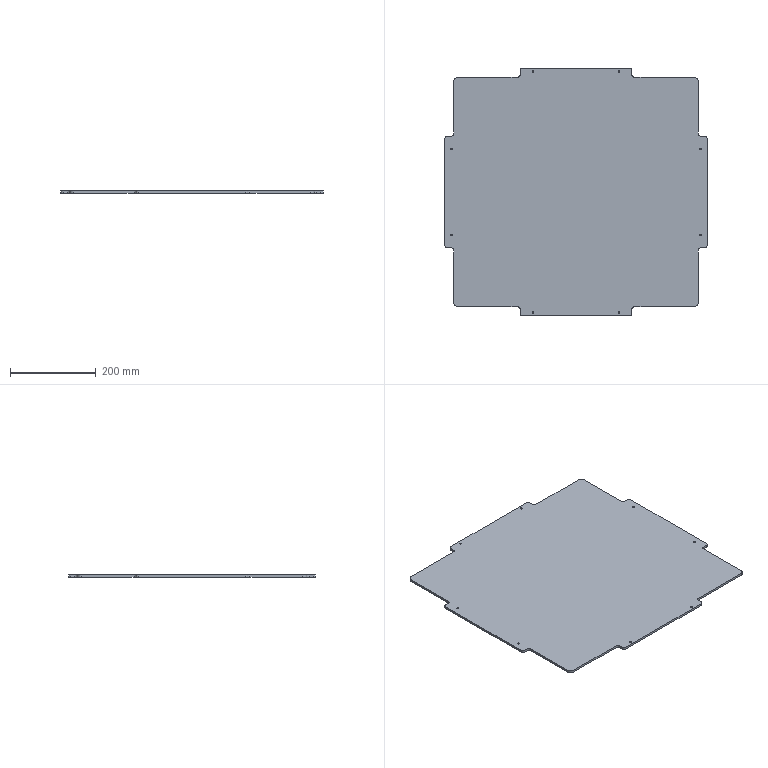Part | SolidWorks | features Fillet 2, ICE 2, Extrusion 1 | 1 solid | 58 faces | box 610 x 575 x 5 mm | volume 1627713 mm3 | cylinder 36 | plane 22 | commonest cylinder face diameters 4.4 x16 10 x16 20 x4